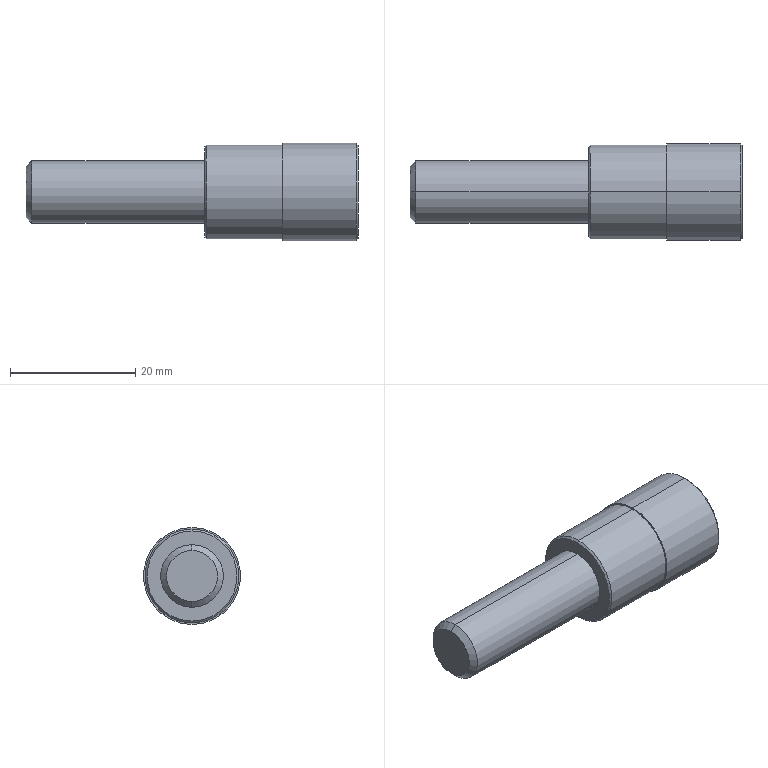Part | SolidWorks | features BaseBody 1 | 1 solid | 34 faces | box 53 x 15.5 x 15.5 mm | volume 5397 mm3 | plane 16 | cone 10 | cylinder 8 | commonest cylinder face diameters 8.376 x2 10 x2 15 x2 15.5 x2
STEP:
#1=CARTESIAN_POINT('',(331.5,35.,40.));
#2=VERTEX_POINT('',#1);
#3=CARTESIAN_POINT('',(331.5,35.,30.));
#4=VERTEX_POINT('',#3);
#5=CARTESIAN_POINT('',(331.5,35.,35.));
#6=DIRECTION('',(-1.,0.,0.));
#7=DIRECTION('',(0.,0.,1.));
#8=AXIS2_PLACEMENT_3D('',#5,#6,#7);
#9=CIRCLE('',#8,5.);
#10=EDGE_CURVE('',#2,#4,#9,.T.);
#11=ORIENTED_EDGE('',*,*,#10,.T.);
#12=CARTESIAN_POINT('',(303.92,35.,30.));
#13=VERTEX_POINT('',#12);
#14=CARTESIAN_POINT('',(317.71,35.,30.));
#15=DIRECTION('',(-1.,0.,0.));
#16=VECTOR('',#15,1000.);
#17=LINE('',#14,#16);
#18=EDGE_CURVE('',#4,#13,#17,.T.);
#19=ORIENTED_EDGE('',*,*,#18,.T.);
#20=CARTESIAN_POINT('',(303.92,35.,40.));
#21=VERTEX_POINT('',#20);
#22=CARTESIAN_POINT('',(303.92,35.,35.));
#23=DIRECTION('',(1.,0.,0.));
#24=DIRECTION('',(0.,0.,1.));
#25=AXIS2_PLACEMENT_3D('',#22,#23,#24);
#26=CIRCLE('',#25,5.);
#27=EDGE_CURVE('',#13,#21,#26,.T.);
#28=ORIENTED_EDGE('',*,*,#27,.T.);
#29=CARTESIAN_POINT('',(317.71,35.,40.));
#30=DIRECTION('',(-1.,0.,0.));
#31=VECTOR('',#30,1000.);
#32=LINE('',#29,#31);
#33=EDGE_CURVE('',#2,#21,#32,.T.);
#34=ORIENTED_EDGE('',*,*,#33,.F.);
#35=EDGE_LOOP('',(#11,#19,#28,#34));
#36=FACE_OUTER_BOUND('',#35,.T.);
#37=CARTESIAN_POINT('',(317.71,35.,35.));
#38=DIRECTION('',(-1.,0.,0.));
#39=DIRECTION('',(0.,0.,1.));
#40=AXIS2_PLACEMENT_3D('',#37,#38,#39);
#41=CYLINDRICAL_SURFACE('',#40,5.);
#42=ADVANCED_FACE('',(#36),#41,.T.);
#43=CARTESIAN_POINT('',(303.,35.,30.92));
#44=VERTEX_POINT('',#43);
#45=CARTESIAN_POINT('',(303.,35.,39.08));
#46=VERTEX_POINT('',#45);
#47=CARTESIAN_POINT('',(303.,35.,35.));
#48=DIRECTION('',(1.,0.,0.));
#49=DIRECTION('',(0.,0.,-1.));
#50=AXIS2_PLACEMENT_3D('',#47,#48,#49);
#51=CIRCLE('',#50,4.08);
#52=EDGE_CURVE('',#44,#46,#51,.T.);
#53=ORIENTED_EDGE('',*,*,#52,.T.);
#54=CARTESIAN_POINT('',(303.92,35.,40.));
#55=DIRECTION('',(0.7071,0.,0.7071));
#56=VECTOR('',#55,1000.);
#57=LINE('',#54,#56);
#58=EDGE_CURVE('',#46,#21,#57,.T.);
#59=ORIENTED_EDGE('',*,*,#58,.T.);
#60=ORIENTED_EDGE('',*,*,#27,.F.);
#61=CARTESIAN_POINT('',(303.92,35.,30.));
#62=DIRECTION('',(0.7071,0.,-0.7071));
#63=VECTOR('',#62,1000.);
#64=LINE('',#61,#63);
#65=EDGE_CURVE('',#44,#13,#64,.T.);
#66=ORIENTED_EDGE('',*,*,#65,.F.);
#67=EDGE_LOOP('',(#53,#59,#60,#66));
#68=FACE_OUTER_BOUND('',#67,.T.);
#69=CARTESIAN_POINT('',(303.92,35.,35.));
#70=DIRECTION('',(1.,0.,0.));
#71=DIRECTION('',(0.,0.,-1.));
#72=AXIS2_PLACEMENT_3D('',#69,#70,#71);
#73=CONICAL_SURFACE('',#72,5.,0.7854);
#74=ADVANCED_FACE('',(#68),#73,.T.);
#75=CARTESIAN_POINT('',(331.5,35.,42.2));
#76=VERTEX_POINT('',#75);
#77=CARTESIAN_POINT('',(331.5,35.,27.8));
#78=VERTEX_POINT('',#77);
#79=CARTESIAN_POINT('',(331.5,35.,35.));
#80=DIRECTION('',(-1.,0.,0.));
#81=DIRECTION('',(0.,0.,-1.));
#82=AXIS2_PLACEMENT_3D('',#79,#80,#81);
#83=CIRCLE('',#82,7.2);
#84=EDGE_CURVE('',#76,#78,#83,.T.);
#85=ORIENTED_EDGE('',*,*,#84,.F.);
#86=CARTESIAN_POINT('',(331.8,35.,42.5));
#87=VERTEX_POINT('',#86);
#88=CARTESIAN_POINT('',(331.8,35.,42.5));
#89=DIRECTION('',(0.7071,0.,0.7071));
#90=VECTOR('',#89,1000.);
#91=LINE('',#88,#90);
#92=EDGE_CURVE('',#76,#87,#91,.T.);
#93=ORIENTED_EDGE('',*,*,#92,.T.);
#94=CARTESIAN_POINT('',(331.8,35.,27.5));
#95=VERTEX_POINT('',#94);
#96=CARTESIAN_POINT('',(331.8,35.,35.));
#97=DIRECTION('',(-1.,0.,0.));
#98=DIRECTION('',(0.,-1.,0.));
#99=AXIS2_PLACEMENT_3D('',#96,#97,#98);
#100=CIRCLE('',#99,7.5);
#101=EDGE_CURVE('',#87,#95,#100,.T.);
#102=ORIENTED_EDGE('',*,*,#101,.T.);
#103=CARTESIAN_POINT('',(331.8,35.,27.5));
#104=DIRECTION('',(0.7071,0.,-0.7071));
#105=VECTOR('',#104,1000.);
#106=LINE('',#103,#105);
#107=EDGE_CURVE('',#78,#95,#106,.T.);
#108=ORIENTED_EDGE('',*,*,#107,.F.);
#109=EDGE_LOOP('',(#85,#93,#102,#108));
#110=FACE_OUTER_BOUND('',#109,.T.);
#111=CARTESIAN_POINT('',(331.8,35.,35.));
#112=DIRECTION('',(1.,0.,0.));
#113=DIRECTION('',(0.,0.,-1.));
#114=AXIS2_PLACEMENT_3D('',#111,#112,#113);
#115=CONICAL_SURFACE('',#114,7.5,0.7854);
#116=ADVANCED_FACE('',(#110),#115,.T.);
#117=CARTESIAN_POINT('',(344.,35.,42.5));
#118=VERTEX_POINT('',#117);
#119=CARTESIAN_POINT('',(344.,35.,27.5));
#120=VERTEX_POINT('',#119);
#121=CARTESIAN_POINT('',(344.,35.,35.));
#122=DIRECTION('',(-1.,0.,0.));
#123=DIRECTION('',(0.,0.,1.));
#124=AXIS2_PLACEMENT_3D('',#121,#122,#123);
#125=CIRCLE('',#124,7.5);
#126=EDGE_CURVE('',#118,#120,#125,.T.);
#127=ORIENTED_EDGE('',*,*,#126,.T.);
#128=CARTESIAN_POINT('',(337.9,35.,27.5));
#129=DIRECTION('',(-1.,0.,0.));
#130=VECTOR('',#129,1000.);
#131=LINE('',#128,#130);
#132=EDGE_CURVE('',#120,#95,#131,.T.);
#133=ORIENTED_EDGE('',*,*,#132,.T.);
#134=ORIENTED_EDGE('',*,*,#101,.F.);
#135=CARTESIAN_POINT('',(337.9,35.,42.5));
#136=DIRECTION('',(-1.,0.,0.));
#137=VECTOR('',#136,1000.);
#138=LINE('',#135,#137);
#139=EDGE_CURVE('',#118,#87,#138,.T.);
#140=ORIENTED_EDGE('',*,*,#139,.F.);
#141=EDGE_LOOP('',(#127,#133,#134,#140));
#142=FACE_OUTER_BOUND('',#141,.T.);
#143=CARTESIAN_POINT('',(337.9,35.,35.));
#144=DIRECTION('',(-1.,0.,0.));
#145=DIRECTION('',(0.,0.,1.));
#146=AXIS2_PLACEMENT_3D('',#143,#144,#145);
#147=CYLINDRICAL_SURFACE('',#146,7.5);
#148=ADVANCED_FACE('',(#142),#147,.T.);
#149=CARTESIAN_POINT('',(355.7,35.,42.75));
#150=VERTEX_POINT('',#149);
#151=CARTESIAN_POINT('',(355.7,35.,27.25));
#152=VERTEX_POINT('',#151);
#153=CARTESIAN_POINT('',(355.7,35.,35.));
#154=DIRECTION('',(-1.,0.,0.));
#155=DIRECTION('',(0.,0.,1.));
#156=AXIS2_PLACEMENT_3D('',#153,#154,#155);
#157=CIRCLE('',#156,7.75);
#158=EDGE_CURVE('',#150,#152,#157,.T.);
#159=ORIENTED_EDGE('',*,*,#158,.T.);
#160=CARTESIAN_POINT('',(344.,35.,27.25));
#161=VERTEX_POINT('',#160);
#162=CARTESIAN_POINT('',(349.85,35.,27.25));
#163=DIRECTION('',(-1.,0.,0.));
#164=VECTOR('',#163,1000.);
#165=LINE('',#162,#164);
#166=EDGE_CURVE('',#152,#161,#165,.T.);
#167=ORIENTED_EDGE('',*,*,#166,.T.);
#168=CARTESIAN_POINT('',(344.,35.,42.75));
#169=VERTEX_POINT('',#168);
#170=CARTESIAN_POINT('',(344.,35.,35.));
#171=DIRECTION('',(-1.,0.,0.));
#172=DIRECTION('',(0.,0.,1.));
#173=AXIS2_PLACEMENT_3D('',#170,#171,#172);
#174=CIRCLE('',#173,7.75);
#175=EDGE_CURVE('',#169,#161,#174,.T.);
#176=ORIENTED_EDGE('',*,*,#175,.F.);
#177=CARTESIAN_POINT('',(349.85,35.,42.75));
#178=DIRECTION('',(-1.,0.,0.));
#179=VECTOR('',#178,1000.);
#180=LINE('',#177,#179);
#181=EDGE_CURVE('',#150,#169,#180,.T.);
#182=ORIENTED_EDGE('',*,*,#181,.F.);
#183=EDGE_LOOP('',(#159,#167,#176,#182));
#184=FACE_OUTER_BOUND('',#183,.T.);
#185=CARTESIAN_POINT('',(349.85,35.,35.));
#186=DIRECTION('',(-1.,0.,0.));
#187=DIRECTION('',(0.,0.,1.));
#188=AXIS2_PLACEMENT_3D('',#185,#186,#187);
#189=CYLINDRICAL_SURFACE('',#188,7.75);
#190=ADVANCED_FACE('',(#184),#189,.T.);
#191=CARTESIAN_POINT('',(356.,35.,42.45));
#192=VERTEX_POINT('',#191);
#193=CARTESIAN_POINT('',(356.,35.,27.55));
#194=VERTEX_POINT('',#193);
#195=CARTESIAN_POINT('',(356.,35.,35.));
#196=DIRECTION('',(-1.,0.,0.));
#197=DIRECTION('',(0.,0.,1.));
#198=AXIS2_PLACEMENT_3D('',#195,#196,#197);
#199=CIRCLE('',#198,7.45);
#200=EDGE_CURVE('',#192,#194,#199,.T.);
#201=ORIENTED_EDGE('',*,*,#200,.T.);
#202=CARTESIAN_POINT('',(355.7,35.,27.25));
#203=DIRECTION('',(-0.7071,0.,-0.7071));
#204=VECTOR('',#203,1000.);
#205=LINE('',#202,#204);
#206=EDGE_CURVE('',#194,#152,#205,.T.);
#207=ORIENTED_EDGE('',*,*,#206,.T.);
#208=ORIENTED_EDGE('',*,*,#158,.F.);
#209=CARTESIAN_POINT('',(355.7,35.,42.75));
#210=DIRECTION('',(-0.7071,0.,0.7071));
#211=VECTOR('',#210,1000.);
#212=LINE('',#209,#211);
#213=EDGE_CURVE('',#192,#150,#212,.T.);
#214=ORIENTED_EDGE('',*,*,#213,.F.);
#215=EDGE_LOOP('',(#201,#207,#208,#214));
#216=FACE_OUTER_BOUND('',#215,.T.);
#217=CARTESIAN_POINT('',(355.7,35.,35.));
#218=DIRECTION('',(-1.,0.,0.));
#219=DIRECTION('',(0.,0.,1.));
#220=AXIS2_PLACEMENT_3D('',#217,#218,#219);
#221=CONICAL_SURFACE('',#220,7.75,0.7854);
#222=ADVANCED_FACE('',(#216),#221,.T.);
#223=CARTESIAN_POINT('',(350.688,35.,39.188));
#224=VERTEX_POINT('',#223);
#225=CARTESIAN_POINT('',(350.688,30.812,35.));
#226=VERTEX_POINT('',#225);
#227=CARTESIAN_POINT('',(350.688,35.,35.));
#228=DIRECTION('',(1.,0.,0.));
#229=DIRECTION('',(0.,-1.,0.));
#230=AXIS2_PLACEMENT_3D('',#227,#228,#229);
#231=CIRCLE('',#230,4.188);
#232=EDGE_CURVE('',#224,#226,#231,.T.);
#233=ORIENTED_EDGE('',*,*,#232,.F.);
#234=CARTESIAN_POINT('',(351.5,35.,40.));
#235=VERTEX_POINT('',#234);
#236=CARTESIAN_POINT('',(351.5,35.,40.));
#237=DIRECTION('',(0.7071,0.,0.7071));
#238=VECTOR('',#237,1000.);
#239=LINE('',#236,#238);
#240=EDGE_CURVE('',#224,#235,#239,.T.);
#241=ORIENTED_EDGE('',*,*,#240,.T.);
#242=CARTESIAN_POINT('',(351.5,30.67,37.5));
#243=VERTEX_POINT('',#242);
#244=CARTESIAN_POINT('',(351.5,35.,35.));
#245=DIRECTION('',(1.,0.,0.));
#246=DIRECTION('',(0.,0.,-1.));
#247=AXIS2_PLACEMENT_3D('',#244,#245,#246);
#248=CIRCLE('',#247,5.);
#249=EDGE_CURVE('',#235,#243,#248,.T.);
#250=ORIENTED_EDGE('',*,*,#249,.T.);
#251=CARTESIAN_POINT('',(351.5,30.67,32.5));
#252=VERTEX_POINT('',#251);
#253=CARTESIAN_POINT('',(351.5,35.,35.));
#254=DIRECTION('',(1.,0.,0.));
#255=DIRECTION('',(0.,0.,-1.));
#256=AXIS2_PLACEMENT_3D('',#253,#254,#255);
#257=CIRCLE('',#256,5.);
#258=EDGE_CURVE('',#243,#252,#257,.T.);
#259=ORIENTED_EDGE('',*,*,#258,.T.);
#260=CARTESIAN_POINT('',(351.5,35.,30.));
#261=VERTEX_POINT('',#260);
#262=CARTESIAN_POINT('',(351.5,35.,35.));
#263=DIRECTION('',(1.,0.,0.));
#264=DIRECTION('',(0.,0.,-1.));
#265=AXIS2_PLACEMENT_3D('',#262,#263,#264);
#266=CIRCLE('',#265,5.);
#267=EDGE_CURVE('',#252,#261,#266,.T.);
#268=ORIENTED_EDGE('',*,*,#267,.T.);
#269=CARTESIAN_POINT('',(350.688,35.,30.812));
#270=VERTEX_POINT('',#269);
#271=CARTESIAN_POINT('',(351.5,35.,30.));
#272=DIRECTION('',(0.7071,0.,-0.7071));
#273=VECTOR('',#272,1000.);
#274=LINE('',#271,#273);
#275=EDGE_CURVE('',#270,#261,#274,.T.);
#276=ORIENTED_EDGE('',*,*,#275,.F.);
#277=CARTESIAN_POINT('',(350.688,35.,35.));
#278=DIRECTION('',(1.,0.,0.));
#279=DIRECTION('',(0.,-1.,0.));
#280=AXIS2_PLACEMENT_3D('',#277,#278,#279);
#281=CIRCLE('',#280,4.188);
#282=EDGE_CURVE('',#226,#270,#281,.T.);
#283=ORIENTED_EDGE('',*,*,#282,.F.);
#284=EDGE_LOOP('',(#233,#241,#250,#259,#268,#276,#283));
#285=FACE_OUTER_BOUND('',#284,.T.);
#286=CARTESIAN_POINT('',(351.5,35.,35.));
#287=DIRECTION('',(1.,0.,0.));
#288=DIRECTION('',(0.,0.,-1.));
#289=AXIS2_PLACEMENT_3D('',#286,#287,#288);
#290=CONICAL_SURFACE('',#289,5.,0.7854);
#291=ADVANCED_FACE('',(#285),#290,.F.);
#292=ORIENTED_EDGE('',*,*,#282,.T.);
#293=CARTESIAN_POINT('',(350.688,39.188,35.));
#294=VERTEX_POINT('',#293);
#295=CARTESIAN_POINT('',(350.688,35.,35.));
#296=DIRECTION('',(1.,0.,0.));
#297=DIRECTION('',(0.,-1.,0.));
#298=AXIS2_PLACEMENT_3D('',#295,#296,#297);
#299=CIRCLE('',#298,4.188);
#300=EDGE_CURVE('',#270,#294,#299,.T.);
#301=ORIENTED_EDGE('',*,*,#300,.T.);
#302=CARTESIAN_POINT('',(336.,39.188,35.));
#303=VERTEX_POINT('',#302);
#304=CARTESIAN_POINT('',(343.344,39.188,35.));
#305=DIRECTION('',(-1.,0.,0.));
#306=VECTOR('',#305,1000.);
#307=LINE('',#304,#306);
#308=EDGE_CURVE('',#294,#303,#307,.T.);
#309=ORIENTED_EDGE('',*,*,#308,.T.);
#310=CARTESIAN_POINT('',(336.,35.,30.812));
#311=VERTEX_POINT('',#310);
#312=CARTESIAN_POINT('',(336.,35.,35.));
#313=DIRECTION('',(1.,0.,0.));
#314=DIRECTION('',(0.,-1.,0.));
#315=AXIS2_PLACEMENT_3D('',#312,#313,#314);
#316=CIRCLE('',#315,4.188);
#317=EDGE_CURVE('',#311,#303,#316,.T.);
#318=ORIENTED_EDGE('',*,*,#317,.F.);
#319=CARTESIAN_POINT('',(336.,30.812,35.));
#320=VERTEX_POINT('',#319);
#321=CARTESIAN_POINT('',(336.,35.,35.));
#322=DIRECTION('',(1.,0.,0.));
#323=DIRECTION('',(0.,-1.,0.));
#324=AXIS2_PLACEMENT_3D('',#321,#322,#323);
#325=CIRCLE('',#324,4.188);
#326=EDGE_CURVE('',#320,#311,#325,.T.);
#327=ORIENTED_EDGE('',*,*,#326,.F.);
#328=CARTESIAN_POINT('',(343.344,30.812,35.));
#329=DIRECTION('',(-1.,0.,0.));
#330=VECTOR('',#329,1000.);
#331=LINE('',#328,#330);
#332=EDGE_CURVE('',#226,#320,#331,.T.);
#333=ORIENTED_EDGE('',*,*,#332,.F.);
#334=EDGE_LOOP('',(#292,#301,#309,#318,#327,#333));
#335=FACE_OUTER_BOUND('',#334,.T.);
#336=CARTESIAN_POINT('',(343.344,35.,35.));
#337=DIRECTION('',(-1.,0.,0.));
#338=DIRECTION('',(0.,-1.,0.));
#339=AXIS2_PLACEMENT_3D('',#336,#337,#338);
#340=CYLINDRICAL_SURFACE('',#339,4.188);
#341=ADVANCED_FACE('',(#335),#340,.F.);
#342=CARTESIAN_POINT('',(333.582,35.,35.));
#343=VERTEX_POINT('',#342);
#344=CARTESIAN_POINT('',(336.,35.,30.812));
#345=DIRECTION('',(0.5,0.,-0.866));
#346=VECTOR('',#345,1000.);
#347=LINE('',#344,#346);
#348=EDGE_CURVE('',#343,#311,#347,.T.);
#349=ORIENTED_EDGE('',*,*,#348,.F.);
#350=CARTESIAN_POINT('',(336.,35.,39.188));
#351=VERTEX_POINT('',#350);
#352=CARTESIAN_POINT('',(336.,35.,39.188));
#353=DIRECTION('',(0.5,0.,0.866));
#354=VECTOR('',#353,1000.);
#355=LINE('',#352,#354);
#356=EDGE_CURVE('',#343,#351,#355,.T.);
#357=ORIENTED_EDGE('',*,*,#356,.T.);
#358=CARTESIAN_POINT('',(336.,35.,35.));
#359=DIRECTION('',(1.,0.,0.));
#360=DIRECTION('',(0.,-1.,0.));
#361=AXIS2_PLACEMENT_3D('',#358,#359,#360);
#362=CIRCLE('',#361,4.188);
#363=EDGE_CURVE('',#351,#320,#362,.T.);
#364=ORIENTED_EDGE('',*,*,#363,.T.);
#365=ORIENTED_EDGE('',*,*,#326,.T.);
#366=EDGE_LOOP('',(#349,#357,#364,#365));
#367=FACE_OUTER_BOUND('',#366,.T.);
#368=CARTESIAN_POINT('',(336.,35.,35.));
#369=DIRECTION('',(1.,0.,0.));
#370=DIRECTION('',(0.,0.,-1.));
#371=AXIS2_PLACEMENT_3D('',#368,#369,#370);
#372=CONICAL_SURFACE('',#371,4.188,1.047);
#373=ADVANCED_FACE('',(#367),#372,.F.);
#374=ORIENTED_EDGE('',*,*,#18,.F.);
#375=CARTESIAN_POINT('',(331.5,35.,35.));
#376=DIRECTION('',(-1.,0.,0.));
#377=DIRECTION('',(0.,0.,1.));
#378=AXIS2_PLACEMENT_3D('',#375,#376,#377);
#379=CIRCLE('',#378,5.);
#380=EDGE_CURVE('',#4,#2,#379,.T.);
#381=ORIENTED_EDGE('',*,*,#380,.T.);
#382=ORIENTED_EDGE('',*,*,#33,.T.);
#383=CARTESIAN_POINT('',(303.92,35.,35.));
#384=DIRECTION('',(1.,0.,0.));
#385=DIRECTION('',(0.,0.,1.));
#386=AXIS2_PLACEMENT_3D('',#383,#384,#385);
#387=CIRCLE('',#386,5.);
#388=EDGE_CURVE('',#21,#13,#387,.T.);
#389=ORIENTED_EDGE('',*,*,#388,.T.);
#390=EDGE_LOOP('',(#374,#381,#382,#389));
#391=FACE_OUTER_BOUND('',#390,.T.);
#392=CARTESIAN_POINT('',(317.71,35.,35.));
#393=DIRECTION('',(-1.,0.,0.));
#394=DIRECTION('',(0.,0.,1.));
#395=AXIS2_PLACEMENT_3D('',#392,#393,#394);
#396=CYLINDRICAL_SURFACE('',#395,5.);
#397=ADVANCED_FACE('',(#391),#396,.T.);
#398=CARTESIAN_POINT('',(331.5,35.,35.));
#399=DIRECTION('',(-1.,0.,0.));
#400=DIRECTION('',(0.,0.,-1.));
#401=AXIS2_PLACEMENT_3D('',#398,#399,#400);
#402=CIRCLE('',#401,7.2);
#403=EDGE_CURVE('',#78,#76,#402,.T.);
#404=ORIENTED_EDGE('',*,*,#403,.T.);
#405=ORIENTED_EDGE('',*,*,#84,.T.);
#406=EDGE_LOOP('',(#404,#405));
#407=FACE_OUTER_BOUND('',#406,.T.);
#408=ORIENTED_EDGE('',*,*,#10,.F.);
#409=ORIENTED_EDGE('',*,*,#380,.F.);
#410=EDGE_LOOP('',(#408,#409));
#411=FACE_BOUND('',#410,.T.);
#412=CARTESIAN_POINT('',(331.5,31.4,35.));
#413=DIRECTION('',(-1.,0.,0.));
#414=DIRECTION('',(0.,0.,1.));
#415=AXIS2_PLACEMENT_3D('',#412,#413,#414);
#416=PLANE('',#415);
#417=ADVANCED_FACE('',(#407,#411),#416,.T.);
#418=ORIENTED_EDGE('',*,*,#58,.F.);
#419=CARTESIAN_POINT('',(303.,35.,35.));
#420=DIRECTION('',(1.,0.,0.));
#421=DIRECTION('',(0.,0.,-1.));
#422=AXIS2_PLACEMENT_3D('',#419,#420,#421);
#423=CIRCLE('',#422,4.08);
#424=EDGE_CURVE('',#46,#44,#423,.T.);
#425=ORIENTED_EDGE('',*,*,#424,.T.);
#426=ORIENTED_EDGE('',*,*,#65,.T.);
#427=ORIENTED_EDGE('',*,*,#388,.F.);
#428=EDGE_LOOP('',(#418,#425,#426,#427));
#429=FACE_OUTER_BOUND('',#428,.T.);
#430=CARTESIAN_POINT('',(303.92,35.,35.));
#431=DIRECTION('',(1.,0.,0.));
#432=DIRECTION('',(0.,0.,-1.));
#433=AXIS2_PLACEMENT_3D('',#430,#431,#432);
#434=CONICAL_SURFACE('',#433,5.,0.7854);
#435=ADVANCED_FACE('',(#429),#434,.T.);
#436=ORIENTED_EDGE('',*,*,#92,.F.);
#437=ORIENTED_EDGE('',*,*,#403,.F.);
#438=ORIENTED_EDGE('',*,*,#107,.T.);
#439=CARTESIAN_POINT('',(331.8,35.,35.));
#440=DIRECTION('',(-1.,0.,0.));
#441=DIRECTION('',(0.,-1.,0.));
#442=AXIS2_PLACEMENT_3D('',#439,#440,#441);
#443=CIRCLE('',#442,7.5);
#444=EDGE_CURVE('',#95,#87,#443,.T.);
#445=ORIENTED_EDGE('',*,*,#444,.T.);
#446=EDGE_LOOP('',(#436,#437,#438,#445));
#447=FACE_OUTER_BOUND('',#446,.T.);
#448=CARTESIAN_POINT('',(331.8,35.,35.));
#449=DIRECTION('',(1.,0.,0.));
#450=DIRECTION('',(0.,0.,-1.));
#451=AXIS2_PLACEMENT_3D('',#448,#449,#450);
#452=CONICAL_SURFACE('',#451,7.5,0.7854);
#453=ADVANCED_FACE('',(#447),#452,.T.);
#454=ORIENTED_EDGE('',*,*,#52,.F.);
#455=ORIENTED_EDGE('',*,*,#424,.F.);
#456=EDGE_LOOP('',(#454,#455));
#457=FACE_OUTER_BOUND('',#456,.T.);
#458=CARTESIAN_POINT('',(303.,32.96,35.));
#459=DIRECTION('',(-1.,0.,0.));
#460=DIRECTION('',(0.,0.,1.));
#461=AXIS2_PLACEMENT_3D('',#458,#459,#460);
#462=PLANE('',#461);
#463=ADVANCED_FACE('',(#457),#462,.T.);
#464=ORIENTED_EDGE('',*,*,#132,.F.);
#465=CARTESIAN_POINT('',(344.,35.,35.));
#466=DIRECTION('',(-1.,0.,0.));
#467=DIRECTION('',(0.,0.,1.));
#468=AXIS2_PLACEMENT_3D('',#465,#466,#467);
#469=CIRCLE('',#468,7.5);
#470=EDGE_CURVE('',#120,#118,#469,.T.);
#471=ORIENTED_EDGE('',*,*,#470,.T.);
#472=ORIENTED_EDGE('',*,*,#139,.T.);
#473=ORIENTED_EDGE('',*,*,#444,.F.);
#474=EDGE_LOOP('',(#464,#471,#472,#473));
#475=FACE_OUTER_BOUND('',#474,.T.);
#476=CARTESIAN_POINT('',(337.9,35.,35.));
#477=DIRECTION('',(-1.,0.,0.));
#478=DIRECTION('',(0.,0.,1.));
#479=AXIS2_PLACEMENT_3D('',#476,#477,#478);
#480=CYLINDRICAL_SURFACE('',#479,7.5);
#481=ADVANCED_FACE('',(#475),#480,.T.);
#482=ORIENTED_EDGE('',*,*,#126,.F.);
#483=ORIENTED_EDGE('',*,*,#470,.F.);
#484=EDGE_LOOP('',(#482,#483));
#485=FACE_BOUND('',#484,.T.);
#486=ORIENTED_EDGE('',*,*,#175,.T.);
#487=CARTESIAN_POINT('',(344.,35.,35.));
#488=DIRECTION('',(-1.,0.,0.));
#489=DIRECTION('',(0.,0.,1.));
#490=AXIS2_PLACEMENT_3D('',#487,#488,#489);
#491=CIRCLE('',#490,7.75);
#492=EDGE_CURVE('',#161,#169,#491,.T.);
#493=ORIENTED_EDGE('',*,*,#492,.T.);
#494=EDGE_LOOP('',(#486,#493));
#495=FACE_OUTER_BOUND('',#494,.T.);
#496=CARTESIAN_POINT('',(344.,27.375,35.));
#497=DIRECTION('',(-1.,0.,0.));
#498=DIRECTION('',(0.,0.,1.));
#499=AXIS2_PLACEMENT_3D('',#496,#497,#498);
#500=PLANE('',#499);
#501=ADVANCED_FACE('',(#485,#495),#500,.T.);
#502=ORIENTED_EDGE('',*,*,#166,.F.);
#503=CARTESIAN_POINT('',(355.7,35.,35.));
#504=DIRECTION('',(-1.,0.,0.));
#505=DIRECTION('',(0.,0.,1.));
#506=AXIS2_PLACEMENT_3D('',#503,#504,#505);
#507=CIRCLE('',#506,7.75);
#508=EDGE_CURVE('',#152,#150,#507,.T.);
#509=ORIENTED_EDGE('',*,*,#508,.T.);
#510=ORIENTED_EDGE('',*,*,#181,.T.);
#511=ORIENTED_EDGE('',*,*,#492,.F.);
#512=EDGE_LOOP('',(#502,#509,#510,#511));
#513=FACE_OUTER_BOUND('',#512,.T.);
#514=CARTESIAN_POINT('',(349.85,35.,35.));
#515=DIRECTION('',(-1.,0.,0.));
#516=DIRECTION('',(0.,0.,1.));
#517=AXIS2_PLACEMENT_3D('',#514,#515,#516);
#518=CYLINDRICAL_SURFACE('',#517,7.75);
#519=ADVANCED_FACE('',(#513),#518,.T.);
#520=ORIENTED_EDGE('',*,*,#206,.F.);
#521=CARTESIAN_POINT('',(356.,35.,35.));
#522=DIRECTION('',(-1.,0.,0.));
#523=DIRECTION('',(0.,0.,1.));
#524=AXIS2_PLACEMENT_3D('',#521,#522,#523);
#525=CIRCLE('',#524,7.45);
#526=EDGE_CURVE('',#194,#192,#525,.T.);
#527=ORIENTED_EDGE('',*,*,#526,.T.);
#528=ORIENTED_EDGE('',*,*,#213,.T.);
#529=ORIENTED_EDGE('',*,*,#508,.F.);
#530=EDGE_LOOP('',(#520,#527,#528,#529));
#531=FACE_OUTER_BOUND('',#530,.T.);
#532=CARTESIAN_POINT('',(355.7,35.,35.));
#533=DIRECTION('',(-1.,0.,0.));
#534=DIRECTION('',(0.,0.,1.));
#535=AXIS2_PLACEMENT_3D('',#532,#533,#534);
#536=CONICAL_SURFACE('',#535,7.75,0.7854);
#537=ADVANCED_FACE('',(#531),#536,.T.);
#538=ORIENTED_EDGE('',*,*,#200,.F.);
#539=ORIENTED_EDGE('',*,*,#526,.F.);
#540=EDGE_LOOP('',(#538,#539));
#541=FACE_OUTER_BOUND('',#540,.T.);
#542=CARTESIAN_POINT('',(356.,37.887,30.));
#543=VERTEX_POINT('',#542);
#544=CARTESIAN_POINT('',(356.,32.113,30.));
#545=VERTEX_POINT('',#544);
#546=CARTESIAN_POINT('',(356.,31.275,30.));
#547=DIRECTION('',(0.,-1.,0.));
#548=VECTOR('',#547,1000.);
#549=LINE('',#546,#548);
#550=EDGE_CURVE('',#543,#545,#549,.T.);
#551=ORIENTED_EDGE('',*,*,#550,.T.);
#552=CARTESIAN_POINT('',(356.,29.226,35.));
#553=VERTEX_POINT('',#552);
#554=CARTESIAN_POINT('',(356.,32.113,30.));
#555=DIRECTION('',(0.,-0.5,0.866));
#556=VECTOR('',#555,1000.);
#557=LINE('',#554,#556);
#558=EDGE_CURVE('',#545,#553,#557,.T.);
#559=ORIENTED_EDGE('',*,*,#558,.T.);
#560=CARTESIAN_POINT('',(356.,32.113,40.));
#561=VERTEX_POINT('',#560);
#562=CARTESIAN_POINT('',(356.,29.226,35.));
#563=DIRECTION('',(0.,0.5,0.866));
#564=VECTOR('',#563,1000.);
#565=LINE('',#562,#564);
#566=EDGE_CURVE('',#553,#561,#565,.T.);
#567=ORIENTED_EDGE('',*,*,#566,.T.);
#568=CARTESIAN_POINT('',(356.,37.887,40.));
#569=VERTEX_POINT('',#568);
#570=CARTESIAN_POINT('',(356.,31.275,40.));
#571=DIRECTION('',(0.,1.,0.));
#572=VECTOR('',#571,1000.);
#573=LINE('',#570,#572);
#574=EDGE_CURVE('',#561,#569,#573,.T.);
#575=ORIENTED_EDGE('',*,*,#574,.T.);
#576=CARTESIAN_POINT('',(356.,40.774,35.));
#577=VERTEX_POINT('',#576);
#578=CARTESIAN_POINT('',(356.,37.887,40.));
#579=DIRECTION('',(0.,0.5,-0.866));
#580=VECTOR('',#579,1000.);
#581=LINE('',#578,#580);
#582=EDGE_CURVE('',#569,#577,#581,.T.);
#583=ORIENTED_EDGE('',*,*,#582,.T.);
#584=CARTESIAN_POINT('',(356.,40.774,35.));
#585=DIRECTION('',(0.,-0.5,-0.866));
#586=VECTOR('',#585,1000.);
#587=LINE('',#584,#586);
#588=EDGE_CURVE('',#577,#543,#587,.T.);
#589=ORIENTED_EDGE('',*,*,#588,.T.);
#590=EDGE_LOOP('',(#551,#559,#567,#575,#583,#589));
#591=FACE_BOUND('',#590,.T.);
#592=CARTESIAN_POINT('',(356.,31.275,35.));
#593=DIRECTION('',(1.,0.,0.));
#594=DIRECTION('',(0.,0.,-1.));
#595=AXIS2_PLACEMENT_3D('',#592,#593,#594);
#596=PLANE('',#595);
#597=ADVANCED_FACE('',(#541,#591),#596,.T.);
#598=CARTESIAN_POINT('',(351.5,29.226,35.));
#599=VERTEX_POINT('',#598);
#600=CARTESIAN_POINT('',(356.,29.226,35.));
#601=DIRECTION('',(-1.,0.,0.));
#602=VECTOR('',#601,1000.);
#603=LINE('',#600,#602);
#604=EDGE_CURVE('',#553,#599,#603,.T.);
#605=ORIENTED_EDGE('',*,*,#604,.F.);
#606=ORIENTED_EDGE('',*,*,#558,.F.);
#607=CARTESIAN_POINT('',(351.5,32.113,30.));
#608=VERTEX_POINT('',#607);
#609=CARTESIAN_POINT('',(356.,32.113,30.));
#610=DIRECTION('',(1.,0.,0.));
#611=VECTOR('',#610,1000.);
#612=LINE('',#609,#611);
#613=EDGE_CURVE('',#608,#545,#612,.T.);
#614=ORIENTED_EDGE('',*,*,#613,.F.);
#615=CARTESIAN_POINT('',(351.5,29.226,35.));
#616=DIRECTION('',(0.,0.5,-0.866));
#617=VECTOR('',#616,1000.);
#618=LINE('',#615,#617);
#619=EDGE_CURVE('',#252,#608,#618,.T.);
#620=ORIENTED_EDGE('',*,*,#619,.F.);
#621=CARTESIAN_POINT('',(351.5,29.226,35.));
#622=DIRECTION('',(0.,0.5,-0.866));
#623=VECTOR('',#622,1000.);
#624=LINE('',#621,#623);
#625=EDGE_CURVE('',#599,#252,#624,.T.);
#626=ORIENTED_EDGE('',*,*,#625,.F.);
#627=EDGE_LOOP('',(#605,#606,#614,#620,#626));
#628=FACE_OUTER_BOUND('',#627,.T.);
#629=CARTESIAN_POINT('',(356.,29.226,35.));
#630=DIRECTION('',(0.,-0.866,-0.5));
#631=DIRECTION('',(0.,0.5,-0.866));
#632=AXIS2_PLACEMENT_3D('',#629,#630,#631);
#633=PLANE('',#632);
#634=ADVANCED_FACE('',(#628),#633,.F.);
#635=ORIENTED_EDGE('',*,*,#613,.T.);
#636=ORIENTED_EDGE('',*,*,#550,.F.);
#637=CARTESIAN_POINT('',(351.5,37.887,30.));
#638=VERTEX_POINT('',#637);
#639=CARTESIAN_POINT('',(356.,37.887,30.));
#640=DIRECTION('',(1.,0.,0.));
#641=VECTOR('',#640,1000.);
#642=LINE('',#639,#641);
#643=EDGE_CURVE('',#638,#543,#642,.T.);
#644=ORIENTED_EDGE('',*,*,#643,.F.);
#645=CARTESIAN_POINT('',(351.5,32.113,30.));
#646=DIRECTION('',(0.,1.,0.));
#647=VECTOR('',#646,1000.);
#648=LINE('',#645,#647);
#649=EDGE_CURVE('',#261,#638,#648,.T.);
#650=ORIENTED_EDGE('',*,*,#649,.F.);
#651=CARTESIAN_POINT('',(351.5,32.113,30.));
#652=DIRECTION('',(0.,1.,0.));
#653=VECTOR('',#652,1000.);
#654=LINE('',#651,#653);
#655=EDGE_CURVE('',#608,#261,#654,.T.);
#656=ORIENTED_EDGE('',*,*,#655,.F.);
#657=EDGE_LOOP('',(#635,#636,#644,#650,#656));
#658=FACE_OUTER_BOUND('',#657,.T.);
#659=CARTESIAN_POINT('',(356.,32.113,30.));
#660=DIRECTION('',(0.,0.,-1.));
#661=DIRECTION('',(-1.,0.,0.));
#662=AXIS2_PLACEMENT_3D('',#659,#660,#661);
#663=PLANE('',#662);
#664=ADVANCED_FACE('',(#658),#663,.F.);
#665=ORIENTED_EDGE('',*,*,#643,.T.);
#666=ORIENTED_EDGE('',*,*,#588,.F.);
#667=CARTESIAN_POINT('',(351.5,40.774,35.));
#668=VERTEX_POINT('',#667);
#669=CARTESIAN_POINT('',(356.,40.774,35.));
#670=DIRECTION('',(1.,0.,0.));
#671=VECTOR('',#670,1000.);
#672=LINE('',#669,#671);
#673=EDGE_CURVE('',#668,#577,#672,.T.);
#674=ORIENTED_EDGE('',*,*,#673,.F.);
#675=CARTESIAN_POINT('',(351.5,39.33,32.5));
#676=VERTEX_POINT('',#675);
#677=CARTESIAN_POINT('',(351.5,37.887,30.));
#678=DIRECTION('',(0.,0.5,0.866));
#679=VECTOR('',#678,1000.);
#680=LINE('',#677,#679);
#681=EDGE_CURVE('',#676,#668,#680,.T.);
#682=ORIENTED_EDGE('',*,*,#681,.F.);
#683=CARTESIAN_POINT('',(351.5,37.887,30.));
#684=DIRECTION('',(0.,0.5,0.866));
#685=VECTOR('',#684,1000.);
#686=LINE('',#683,#685);
#687=EDGE_CURVE('',#638,#676,#686,.T.);
#688=ORIENTED_EDGE('',*,*,#687,.F.);
#689=EDGE_LOOP('',(#665,#666,#674,#682,#688));
#690=FACE_OUTER_BOUND('',#689,.T.);
#691=CARTESIAN_POINT('',(356.,37.887,30.));
#692=DIRECTION('',(0.,0.866,-0.5));
#693=DIRECTION('',(0.,0.5,0.866));
#694=AXIS2_PLACEMENT_3D('',#691,#692,#693);
#695=PLANE('',#694);
#696=ADVANCED_FACE('',(#690),#695,.F.);
#697=ORIENTED_EDGE('',*,*,#673,.T.);
#698=ORIENTED_EDGE('',*,*,#582,.F.);
#699=CARTESIAN_POINT('',(351.5,37.887,40.));
#700=VERTEX_POINT('',#699);
#701=CARTESIAN_POINT('',(356.,37.887,40.));
#702=DIRECTION('',(1.,0.,0.));
#703=VECTOR('',#702,1000.);
#704=LINE('',#701,#703);
#705=EDGE_CURVE('',#700,#569,#704,.T.);
#706=ORIENTED_EDGE('',*,*,#705,.F.);
#707=CARTESIAN_POINT('',(351.5,39.33,37.5));
#708=VERTEX_POINT('',#707);
#709=CARTESIAN_POINT('',(351.5,40.774,35.));
#710=DIRECTION('',(0.,-0.5,0.866));
#711=VECTOR('',#710,1000.);
#712=LINE('',#709,#711);
#713=EDGE_CURVE('',#708,#700,#712,.T.);
#714=ORIENTED_EDGE('',*,*,#713,.F.);
#715=CARTESIAN_POINT('',(351.5,40.774,35.));
#716=DIRECTION('',(0.,-0.5,0.866));
#717=VECTOR('',#716,1000.);
#718=LINE('',#715,#717);
#719=EDGE_CURVE('',#668,#708,#718,.T.);
#720=ORIENTED_EDGE('',*,*,#719,.F.);
#721=EDGE_LOOP('',(#697,#698,#706,#714,#720));
#722=FACE_OUTER_BOUND('',#721,.T.);
#723=CARTESIAN_POINT('',(356.,40.774,35.));
#724=DIRECTION('',(0.,0.866,0.5));
#725=DIRECTION('',(0.,-0.5,0.866));
#726=AXIS2_PLACEMENT_3D('',#723,#724,#725);
#727=PLANE('',#726);
#728=ADVANCED_FACE('',(#722),#727,.F.);
#729=ORIENTED_EDGE('',*,*,#705,.T.);
#730=ORIENTED_EDGE('',*,*,#574,.F.);
#731=CARTESIAN_POINT('',(351.5,32.113,40.));
#732=VERTEX_POINT('',#731);
#733=CARTESIAN_POINT('',(356.,32.113,40.));
#734=DIRECTION('',(1.,0.,0.));
#735=VECTOR('',#734,1000.);
#736=LINE('',#733,#735);
#737=EDGE_CURVE('',#732,#561,#736,.T.);
#738=ORIENTED_EDGE('',*,*,#737,.F.);
#739=CARTESIAN_POINT('',(351.5,37.887,40.));
#740=DIRECTION('',(0.,-1.,0.));
#741=VECTOR('',#740,1000.);
#742=LINE('',#739,#741);
#743=EDGE_CURVE('',#235,#732,#742,.T.);
#744=ORIENTED_EDGE('',*,*,#743,.F.);
#745=CARTESIAN_POINT('',(351.5,37.887,40.));
#746=DIRECTION('',(0.,-1.,0.));
#747=VECTOR('',#746,1000.);
#748=LINE('',#745,#747);
#749=EDGE_CURVE('',#700,#235,#748,.T.);
#750=ORIENTED_EDGE('',*,*,#749,.F.);
#751=EDGE_LOOP('',(#729,#730,#738,#744,#750));
#752=FACE_OUTER_BOUND('',#751,.T.);
#753=CARTESIAN_POINT('',(356.,37.887,40.));
#754=DIRECTION('',(0.,0.,1.));
#755=DIRECTION('',(1.,0.,0.));
#756=AXIS2_PLACEMENT_3D('',#753,#754,#755);
#757=PLANE('',#756);
#758=ADVANCED_FACE('',(#752),#757,.F.);
#759=ORIENTED_EDGE('',*,*,#737,.T.);
#760=ORIENTED_EDGE('',*,*,#566,.F.);
#761=ORIENTED_EDGE('',*,*,#604,.T.);
#762=CARTESIAN_POINT('',(351.5,32.113,40.));
#763=DIRECTION('',(0.,-0.5,-0.866));
#764=VECTOR('',#763,1000.);
#765=LINE('',#762,#764);
#766=EDGE_CURVE('',#243,#599,#765,.T.);
#767=ORIENTED_EDGE('',*,*,#766,.F.);
#768=CARTESIAN_POINT('',(351.5,32.113,40.));
#769=DIRECTION('',(0.,-0.5,-0.866));
#770=VECTOR('',#769,1000.);
#771=LINE('',#768,#770);
#772=EDGE_CURVE('',#732,#243,#771,.T.);
#773=ORIENTED_EDGE('',*,*,#772,.F.);
#774=EDGE_LOOP('',(#759,#760,#761,#767,#773));
#775=FACE_OUTER_BOUND('',#774,.T.);
#776=CARTESIAN_POINT('',(356.,32.113,40.));
#777=DIRECTION('',(0.,-0.866,0.5));
#778=DIRECTION('',(0.,-0.5,-0.866));
#779=AXIS2_PLACEMENT_3D('',#776,#777,#778);
#780=PLANE('',#779);
#781=ADVANCED_FACE('',(#775),#780,.F.);
#782=ORIENTED_EDGE('',*,*,#258,.F.);
#783=ORIENTED_EDGE('',*,*,#766,.T.);
#784=ORIENTED_EDGE('',*,*,#625,.T.);
#785=EDGE_LOOP('',(#782,#783,#784));
#786=FACE_OUTER_BOUND('',#785,.T.);
#787=CARTESIAN_POINT('',(351.5,35.,35.));
#788=DIRECTION('',(-1.,0.,0.));
#789=DIRECTION('',(0.,0.,1.));
#790=AXIS2_PLACEMENT_3D('',#787,#788,#789);
#791=PLANE('',#790);
#792=ADVANCED_FACE('',(#786),#791,.F.);
#793=ORIENTED_EDGE('',*,*,#619,.T.);
#794=ORIENTED_EDGE('',*,*,#655,.T.);
#795=ORIENTED_EDGE('',*,*,#267,.F.);
#796=EDGE_LOOP('',(#793,#794,#795));
#797=FACE_OUTER_BOUND('',#796,.T.);
#798=CARTESIAN_POINT('',(351.5,35.,35.));
#799=DIRECTION('',(-1.,0.,0.));
#800=DIRECTION('',(0.,0.,1.));
#801=AXIS2_PLACEMENT_3D('',#798,#799,#800);
#802=PLANE('',#801);
#803=ADVANCED_FACE('',(#797),#802,.F.);
#804=ORIENTED_EDGE('',*,*,#649,.T.);
#805=ORIENTED_EDGE('',*,*,#687,.T.);
#806=CARTESIAN_POINT('',(351.5,35.,35.));
#807=DIRECTION('',(1.,0.,0.));
#808=DIRECTION('',(0.,0.,-1.));
#809=AXIS2_PLACEMENT_3D('',#806,#807,#808);
#810=CIRCLE('',#809,5.);
#811=EDGE_CURVE('',#261,#676,#810,.T.);
#812=ORIENTED_EDGE('',*,*,#811,.F.);
#813=EDGE_LOOP('',(#804,#805,#812));
#814=FACE_OUTER_BOUND('',#813,.T.);
#815=CARTESIAN_POINT('',(351.5,35.,35.));
#816=DIRECTION('',(-1.,0.,0.));
#817=DIRECTION('',(0.,0.,1.));
#818=AXIS2_PLACEMENT_3D('',#815,#816,#817);
#819=PLANE('',#818);
#820=ADVANCED_FACE('',(#814),#819,.F.);
#821=CARTESIAN_POINT('',(351.5,35.,35.));
#822=DIRECTION('',(1.,0.,0.));
#823=DIRECTION('',(0.,0.,-1.));
#824=AXIS2_PLACEMENT_3D('',#821,#822,#823);
#825=CIRCLE('',#824,5.);
#826=EDGE_CURVE('',#676,#708,#825,.T.);
#827=ORIENTED_EDGE('',*,*,#826,.F.);
#828=ORIENTED_EDGE('',*,*,#681,.T.);
#829=ORIENTED_EDGE('',*,*,#719,.T.);
#830=EDGE_LOOP('',(#827,#828,#829));
#831=FACE_OUTER_BOUND('',#830,.T.);
#832=CARTESIAN_POINT('',(351.5,35.,35.));
#833=DIRECTION('',(-1.,0.,0.));
#834=DIRECTION('',(0.,0.,1.));
#835=AXIS2_PLACEMENT_3D('',#832,#833,#834);
#836=PLANE('',#835);
#837=ADVANCED_FACE('',(#831),#836,.F.);
#838=ORIENTED_EDGE('',*,*,#713,.T.);
#839=ORIENTED_EDGE('',*,*,#749,.T.);
#840=CARTESIAN_POINT('',(351.5,35.,35.));
#841=DIRECTION('',(1.,0.,0.));
#842=DIRECTION('',(0.,0.,-1.));
#843=AXIS2_PLACEMENT_3D('',#840,#841,#842);
#844=CIRCLE('',#843,5.);
#845=EDGE_CURVE('',#708,#235,#844,.T.);
#846=ORIENTED_EDGE('',*,*,#845,.F.);
#847=EDGE_LOOP('',(#838,#839,#846));
#848=FACE_OUTER_BOUND('',#847,.T.);
#849=CARTESIAN_POINT('',(351.5,35.,35.));
#850=DIRECTION('',(-1.,0.,0.));
#851=DIRECTION('',(0.,0.,1.));
#852=AXIS2_PLACEMENT_3D('',#849,#850,#851);
#853=PLANE('',#852);
#854=ADVANCED_FACE('',(#848),#853,.F.);
#855=ORIENTED_EDGE('',*,*,#743,.T.);
#856=ORIENTED_EDGE('',*,*,#772,.T.);
#857=ORIENTED_EDGE('',*,*,#249,.F.);
#858=EDGE_LOOP('',(#855,#856,#857));
#859=FACE_OUTER_BOUND('',#858,.T.);
#860=CARTESIAN_POINT('',(351.5,35.,35.));
#861=DIRECTION('',(-1.,0.,0.));
#862=DIRECTION('',(0.,0.,1.));
#863=AXIS2_PLACEMENT_3D('',#860,#861,#862);
#864=PLANE('',#863);
#865=ADVANCED_FACE('',(#859),#864,.F.);
#866=ORIENTED_EDGE('',*,*,#240,.F.);
#867=CARTESIAN_POINT('',(350.688,35.,35.));
#868=DIRECTION('',(1.,0.,0.));
#869=DIRECTION('',(0.,-1.,0.));
#870=AXIS2_PLACEMENT_3D('',#867,#868,#869);
#871=CIRCLE('',#870,4.188);
#872=EDGE_CURVE('',#294,#224,#871,.T.);
#873=ORIENTED_EDGE('',*,*,#872,.F.);
#874=ORIENTED_EDGE('',*,*,#300,.F.);
#875=ORIENTED_EDGE('',*,*,#275,.T.);
#876=ORIENTED_EDGE('',*,*,#811,.T.);
#877=ORIENTED_EDGE('',*,*,#826,.T.);
#878=ORIENTED_EDGE('',*,*,#845,.T.);
#879=EDGE_LOOP('',(#866,#873,#874,#875,#876,#877,#878));
#880=FACE_OUTER_BOUND('',#879,.T.);
#881=CARTESIAN_POINT('',(351.5,35.,35.));
#882=DIRECTION('',(1.,0.,0.));
#883=DIRECTION('',(0.,0.,-1.));
#884=AXIS2_PLACEMENT_3D('',#881,#882,#883);
#885=CONICAL_SURFACE('',#884,5.,0.7854);
#886=ADVANCED_FACE('',(#880),#885,.F.);
#887=ORIENTED_EDGE('',*,*,#308,.F.);
#888=ORIENTED_EDGE('',*,*,#872,.T.);
#889=ORIENTED_EDGE('',*,*,#232,.T.);
#890=ORIENTED_EDGE('',*,*,#332,.T.);
#891=ORIENTED_EDGE('',*,*,#363,.F.);
#892=CARTESIAN_POINT('',(336.,35.,35.));
#893=DIRECTION('',(1.,0.,0.));
#894=DIRECTION('',(0.,-1.,0.));
#895=AXIS2_PLACEMENT_3D('',#892,#893,#894);
#896=CIRCLE('',#895,4.188);
#897=EDGE_CURVE('',#303,#351,#896,.T.);
#898=ORIENTED_EDGE('',*,*,#897,.F.);
#899=EDGE_LOOP('',(#887,#888,#889,#890,#891,#898));
#900=FACE_OUTER_BOUND('',#899,.T.);
#901=CARTESIAN_POINT('',(343.344,35.,35.));
#902=DIRECTION('',(-1.,0.,0.));
#903=DIRECTION('',(0.,-1.,0.));
#904=AXIS2_PLACEMENT_3D('',#901,#902,#903);
#905=CYLINDRICAL_SURFACE('',#904,4.188);
#906=ADVANCED_FACE('',(#900),#905,.F.);
#907=ORIENTED_EDGE('',*,*,#356,.F.);
#908=ORIENTED_EDGE('',*,*,#348,.T.);
#909=ORIENTED_EDGE('',*,*,#317,.T.);
#910=ORIENTED_EDGE('',*,*,#897,.T.);
#911=EDGE_LOOP('',(#907,#908,#909,#910));
#912=FACE_OUTER_BOUND('',#911,.T.);
#913=CARTESIAN_POINT('',(336.,35.,35.));
#914=DIRECTION('',(1.,0.,0.));
#915=DIRECTION('',(0.,0.,-1.));
#916=AXIS2_PLACEMENT_3D('',#913,#914,#915);
#917=CONICAL_SURFACE('',#916,4.188,1.047);
#918=ADVANCED_FACE('',(#912),#917,.F.);
#919=CLOSED_SHELL('',(#42,#74,#116,#148,#190,#222,#291,#341,#373,#397,#417,#435,#453,#463,#481,#501,#519,#537,#597,#634,#664,#696,#728,#758,#781,#792,#803,#820,#837,#854,#865,#886,#906,#918));
#920=MANIFOLD_SOLID_BREP('',#919);
#921=CARTESIAN_POINT('',(0.,0.,0.));
#922=DIRECTION('',(0.,0.,1.));
#923=DIRECTION('',(1.,0.,0.));
#924=AXIS2_PLACEMENT_3D('',#921,#922,#923);
#925=(LENGTH_UNIT()NAMED_UNIT(*)SI_UNIT(.MILLI.,.METRE.));
#926=UNCERTAINTY_MEASURE_WITH_UNIT(LENGTH_MEASURE(0.00001),#925,'','');
#927=(NAMED_UNIT(*)PLANE_ANGLE_UNIT()SI_UNIT($,.RADIAN.));
#928=(NAMED_UNIT(*)SI_UNIT($,.STERADIAN.)SOLID_ANGLE_UNIT());
#929=(GEOMETRIC_REPRESENTATION_CONTEXT(3)GLOBAL_UNCERTAINTY_ASSIGNED_CONTEXT((#926))GLOBAL_UNIT_ASSIGNED_CONTEXT((#925,#927,#928))REPRESENTATION_CONTEXT('',''));
#930=ADVANCED_BREP_SHAPE_REPRESENTATION('',(#920,#924),#929);